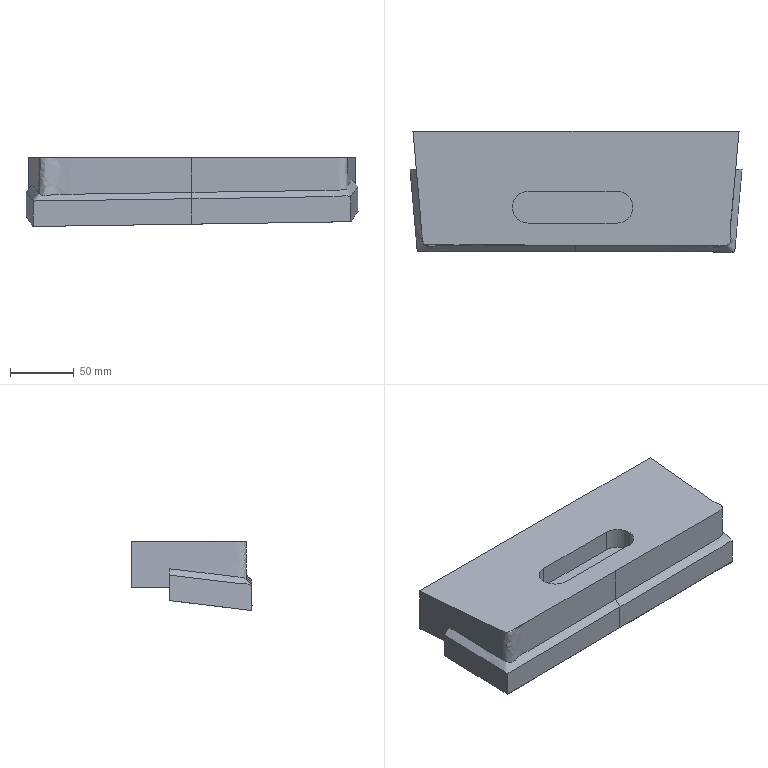Part | NX | features solid 2 | 1 solid | 40 faces | box 261.433 x 95.053 x 54.076 mm | volume 750636 mm3 | plane 17 | spline 16 | cylinder 7 | commonest cylinder face diameters 30 x5 25 x2